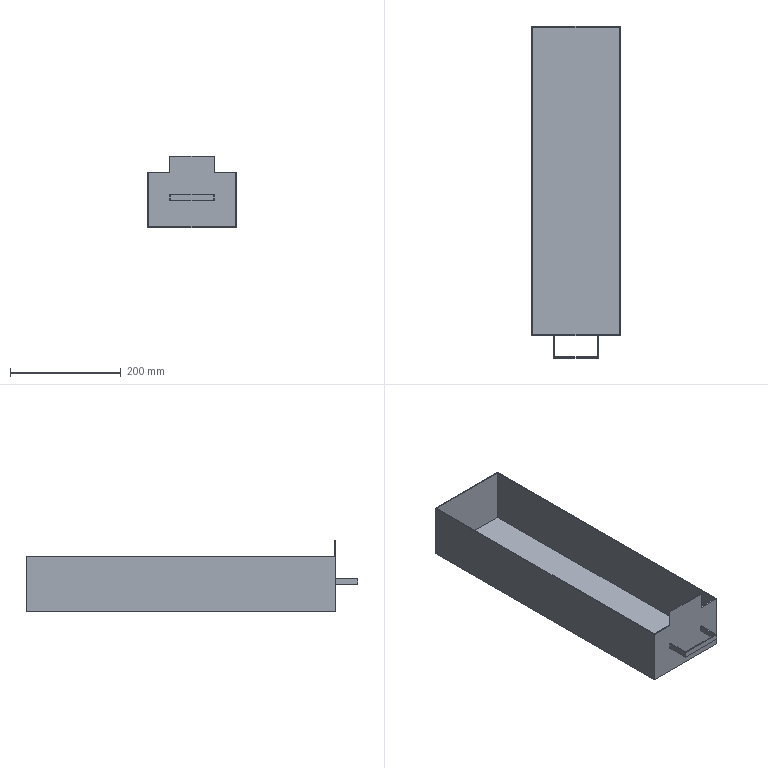Part | NX | features solid 2 | 1 solid | 22 faces | box 160 x 600 x 130 mm | volume 467792 mm3 | plane 22
STEP:
#1=CARTESIAN_POINT('',(375.,-427.,-465.));
#2=VERTEX_POINT('',#1);
#3=CARTESIAN_POINT('',(375.,-987.,-465.));
#4=VERTEX_POINT('',#3);
#5=CARTESIAN_POINT('',(375.,-687.,-465.));
#6=DIRECTION('',(0.,-1.,0.));
#7=VECTOR('',#6,1000.);
#8=LINE('',#5,#7);
#9=EDGE_CURVE('',#2,#4,#8,.T.);
#10=ORIENTED_EDGE('',*,*,#9,.T.);
#11=CARTESIAN_POINT('',(375.,-987.,-565.));
#12=VERTEX_POINT('',#11);
#13=CARTESIAN_POINT('',(375.,-987.,-565.));
#14=DIRECTION('',(0.,0.,1.));
#15=VECTOR('',#14,1000.);
#16=LINE('',#13,#15);
#17=EDGE_CURVE('',#12,#4,#16,.T.);
#18=ORIENTED_EDGE('',*,*,#17,.F.);
#19=CARTESIAN_POINT('',(375.,-427.,-565.));
#20=VERTEX_POINT('',#19);
#21=CARTESIAN_POINT('',(375.,-687.,-565.));
#22=DIRECTION('',(0.,-1.,0.));
#23=VECTOR('',#22,1000.);
#24=LINE('',#21,#23);
#25=EDGE_CURVE('',#20,#12,#24,.T.);
#26=ORIENTED_EDGE('',*,*,#25,.F.);
#27=CARTESIAN_POINT('',(375.,-427.,-565.));
#28=DIRECTION('',(0.,0.,-1.));
#29=VECTOR('',#28,1000.);
#30=LINE('',#27,#29);
#31=EDGE_CURVE('',#20,#2,#30,.F.);
#32=ORIENTED_EDGE('',*,*,#31,.T.);
#33=EDGE_LOOP('',(#10,#18,#26,#32));
#34=FACE_BOUND('',#33,.T.);
#35=CARTESIAN_POINT('',(375.,-687.,-565.));
#36=DIRECTION('',(-1.,0.,0.));
#37=DIRECTION('',(0.,-1.,0.));
#38=AXIS2_PLACEMENT_3D('',#35,#36,#37);
#39=PLANE('',#38);
#40=ADVANCED_FACE('',(#34),#39,.F.);
#41=CARTESIAN_POINT('',(255.,-987.,-505.));
#42=VERTEX_POINT('',#41);
#43=CARTESIAN_POINT('',(255.,-987.,-515.));
#44=VERTEX_POINT('',#43);
#45=CARTESIAN_POINT('',(255.,-987.,-565.));
#46=DIRECTION('',(0.,0.,-1.));
#47=VECTOR('',#46,1000.);
#48=LINE('',#45,#47);
#49=EDGE_CURVE('',#42,#44,#48,.T.);
#50=ORIENTED_EDGE('',*,*,#49,.F.);
#51=CARTESIAN_POINT('',(257.,-987.,-505.));
#52=VERTEX_POINT('',#51);
#53=CARTESIAN_POINT('',(335.,-987.,-505.));
#54=DIRECTION('',(1.,0.,0.));
#55=VECTOR('',#54,1000.);
#56=LINE('',#53,#55);
#57=EDGE_CURVE('',#52,#42,#56,.F.);
#58=ORIENTED_EDGE('',*,*,#57,.F.);
#59=CARTESIAN_POINT('',(257.,-987.,-515.));
#60=VERTEX_POINT('',#59);
#61=CARTESIAN_POINT('',(257.,-987.,-565.));
#62=DIRECTION('',(0.,0.,-1.));
#63=VECTOR('',#62,1000.);
#64=LINE('',#61,#63);
#65=EDGE_CURVE('',#52,#60,#64,.T.);
#66=ORIENTED_EDGE('',*,*,#65,.T.);
#67=CARTESIAN_POINT('',(335.,-987.,-515.));
#68=DIRECTION('',(1.,0.,0.));
#69=VECTOR('',#68,1000.);
#70=LINE('',#67,#69);
#71=EDGE_CURVE('',#60,#44,#70,.F.);
#72=ORIENTED_EDGE('',*,*,#71,.T.);
#73=EDGE_LOOP('',(#50,#58,#66,#72));
#74=FACE_BOUND('',#73,.T.);
#75=CARTESIAN_POINT('',(333.,-987.,-505.));
#76=VERTEX_POINT('',#75);
#77=CARTESIAN_POINT('',(333.,-987.,-515.));
#78=VERTEX_POINT('',#77);
#79=CARTESIAN_POINT('',(333.,-987.,-565.));
#80=DIRECTION('',(0.,0.,1.));
#81=VECTOR('',#80,1000.);
#82=LINE('',#79,#81);
#83=EDGE_CURVE('',#76,#78,#82,.F.);
#84=ORIENTED_EDGE('',*,*,#83,.F.);
#85=CARTESIAN_POINT('',(335.,-987.,-505.));
#86=VERTEX_POINT('',#85);
#87=CARTESIAN_POINT('',(335.,-987.,-505.));
#88=DIRECTION('',(1.,0.,0.));
#89=VECTOR('',#88,1000.);
#90=LINE('',#87,#89);
#91=EDGE_CURVE('',#86,#76,#90,.F.);
#92=ORIENTED_EDGE('',*,*,#91,.F.);
#93=CARTESIAN_POINT('',(335.,-987.,-515.));
#94=VERTEX_POINT('',#93);
#95=CARTESIAN_POINT('',(335.,-987.,-565.));
#96=DIRECTION('',(0.,0.,-1.));
#97=VECTOR('',#96,1000.);
#98=LINE('',#95,#97);
#99=EDGE_CURVE('',#86,#94,#98,.T.);
#100=ORIENTED_EDGE('',*,*,#99,.T.);
#101=CARTESIAN_POINT('',(335.,-987.,-515.));
#102=DIRECTION('',(1.,0.,0.));
#103=VECTOR('',#102,1000.);
#104=LINE('',#101,#103);
#105=EDGE_CURVE('',#94,#78,#104,.F.);
#106=ORIENTED_EDGE('',*,*,#105,.T.);
#107=EDGE_LOOP('',(#84,#92,#100,#106));
#108=FACE_BOUND('',#107,.T.);
#109=CARTESIAN_POINT('',(215.,-987.,-465.));
#110=VERTEX_POINT('',#109);
#111=CARTESIAN_POINT('',(255.,-987.,-465.));
#112=VERTEX_POINT('',#111);
#113=CARTESIAN_POINT('',(370.,-987.,-465.));
#114=DIRECTION('',(1.,0.,0.));
#115=VECTOR('',#114,1000.);
#116=LINE('',#113,#115);
#117=EDGE_CURVE('',#110,#112,#116,.T.);
#118=ORIENTED_EDGE('',*,*,#117,.F.);
#119=CARTESIAN_POINT('',(215.,-987.,-565.));
#120=VERTEX_POINT('',#119);
#121=CARTESIAN_POINT('',(215.,-987.,-565.));
#122=DIRECTION('',(0.,0.,-1.));
#123=VECTOR('',#122,1000.);
#124=LINE('',#121,#123);
#125=EDGE_CURVE('',#120,#110,#124,.F.);
#126=ORIENTED_EDGE('',*,*,#125,.F.);
#127=CARTESIAN_POINT('',(370.,-987.,-565.));
#128=DIRECTION('',(-1.,0.,0.));
#129=VECTOR('',#128,1000.);
#130=LINE('',#127,#129);
#131=EDGE_CURVE('',#12,#120,#130,.T.);
#132=ORIENTED_EDGE('',*,*,#131,.F.);
#133=ORIENTED_EDGE('',*,*,#17,.T.);
#134=CARTESIAN_POINT('',(335.,-987.,-465.));
#135=VERTEX_POINT('',#134);
#136=CARTESIAN_POINT('',(370.,-987.,-465.));
#137=DIRECTION('',(1.,0.,0.));
#138=VECTOR('',#137,1000.);
#139=LINE('',#136,#138);
#140=EDGE_CURVE('',#135,#4,#139,.T.);
#141=ORIENTED_EDGE('',*,*,#140,.F.);
#142=CARTESIAN_POINT('',(335.,-987.,-435.));
#143=VERTEX_POINT('',#142);
#144=CARTESIAN_POINT('',(335.,-987.,-565.));
#145=DIRECTION('',(0.,0.,1.));
#146=VECTOR('',#145,1000.);
#147=LINE('',#144,#146);
#148=EDGE_CURVE('',#135,#143,#147,.T.);
#149=ORIENTED_EDGE('',*,*,#148,.T.);
#150=CARTESIAN_POINT('',(255.,-987.,-435.));
#151=VERTEX_POINT('',#150);
#152=CARTESIAN_POINT('',(375.,-987.,-435.));
#153=DIRECTION('',(-1.,0.,0.));
#154=VECTOR('',#153,1000.);
#155=LINE('',#152,#154);
#156=EDGE_CURVE('',#143,#151,#155,.T.);
#157=ORIENTED_EDGE('',*,*,#156,.T.);
#158=CARTESIAN_POINT('',(255.,-987.,-565.));
#159=DIRECTION('',(0.,0.,-1.));
#160=VECTOR('',#159,1000.);
#161=LINE('',#158,#160);
#162=EDGE_CURVE('',#112,#151,#161,.F.);
#163=ORIENTED_EDGE('',*,*,#162,.F.);
#164=EDGE_LOOP('',(#118,#126,#132,#133,#141,#149,#157,#163));
#165=FACE_BOUND('',#164,.T.);
#166=CARTESIAN_POINT('',(370.,-987.,-565.));
#167=DIRECTION('',(0.,1.,0.));
#168=DIRECTION('',(-1.,0.,0.));
#169=AXIS2_PLACEMENT_3D('',#166,#167,#168);
#170=PLANE('',#169);
#171=ADVANCED_FACE('',(#74,#108,#165),#170,.F.);
#172=ORIENTED_EDGE('',*,*,#125,.T.);
#173=CARTESIAN_POINT('',(215.,-427.,-465.));
#174=VERTEX_POINT('',#173);
#175=CARTESIAN_POINT('',(215.,-687.,-465.));
#176=DIRECTION('',(0.,1.,0.));
#177=VECTOR('',#176,1000.);
#178=LINE('',#175,#177);
#179=EDGE_CURVE('',#174,#110,#178,.F.);
#180=ORIENTED_EDGE('',*,*,#179,.F.);
#181=CARTESIAN_POINT('',(215.,-427.,-565.));
#182=VERTEX_POINT('',#181);
#183=CARTESIAN_POINT('',(215.,-427.,-565.));
#184=DIRECTION('',(0.,0.,1.));
#185=VECTOR('',#184,1000.);
#186=LINE('',#183,#185);
#187=EDGE_CURVE('',#182,#174,#186,.T.);
#188=ORIENTED_EDGE('',*,*,#187,.F.);
#189=CARTESIAN_POINT('',(215.,-687.,-565.));
#190=DIRECTION('',(0.,1.,0.));
#191=VECTOR('',#190,1000.);
#192=LINE('',#189,#191);
#193=EDGE_CURVE('',#182,#120,#192,.F.);
#194=ORIENTED_EDGE('',*,*,#193,.T.);
#195=EDGE_LOOP('',(#172,#180,#188,#194));
#196=FACE_BOUND('',#195,.T.);
#197=CARTESIAN_POINT('',(215.,-687.,-565.));
#198=DIRECTION('',(-1.,0.,0.));
#199=DIRECTION('',(0.,-1.,0.));
#200=AXIS2_PLACEMENT_3D('',#197,#198,#199);
#201=PLANE('',#200);
#202=ADVANCED_FACE('',(#196),#201,.T.);
#203=CARTESIAN_POINT('',(217.,-985.,-563.));
#204=VERTEX_POINT('',#203);
#205=CARTESIAN_POINT('',(217.,-985.,-465.));
#206=VERTEX_POINT('',#205);
#207=CARTESIAN_POINT('',(217.,-985.,-565.));
#208=DIRECTION('',(0.,0.,-1.));
#209=VECTOR('',#208,1000.);
#210=LINE('',#207,#209);
#211=EDGE_CURVE('',#204,#206,#210,.F.);
#212=ORIENTED_EDGE('',*,*,#211,.T.);
#213=CARTESIAN_POINT('',(255.,-985.,-465.));
#214=VERTEX_POINT('',#213);
#215=CARTESIAN_POINT('',(370.,-985.,-465.));
#216=DIRECTION('',(1.,0.,0.));
#217=VECTOR('',#216,1000.);
#218=LINE('',#215,#217);
#219=EDGE_CURVE('',#206,#214,#218,.T.);
#220=ORIENTED_EDGE('',*,*,#219,.T.);
#221=CARTESIAN_POINT('',(255.,-985.,-435.));
#222=VERTEX_POINT('',#221);
#223=CARTESIAN_POINT('',(255.,-985.,-565.));
#224=DIRECTION('',(0.,0.,-1.));
#225=VECTOR('',#224,1000.);
#226=LINE('',#223,#225);
#227=EDGE_CURVE('',#214,#222,#226,.F.);
#228=ORIENTED_EDGE('',*,*,#227,.T.);
#229=CARTESIAN_POINT('',(335.,-985.,-435.));
#230=VERTEX_POINT('',#229);
#231=CARTESIAN_POINT('',(375.,-985.,-435.));
#232=DIRECTION('',(-1.,0.,0.));
#233=VECTOR('',#232,1000.);
#234=LINE('',#231,#233);
#235=EDGE_CURVE('',#230,#222,#234,.T.);
#236=ORIENTED_EDGE('',*,*,#235,.F.);
#237=CARTESIAN_POINT('',(335.,-985.,-465.));
#238=VERTEX_POINT('',#237);
#239=CARTESIAN_POINT('',(335.,-985.,-565.));
#240=DIRECTION('',(0.,0.,1.));
#241=VECTOR('',#240,1000.);
#242=LINE('',#239,#241);
#243=EDGE_CURVE('',#238,#230,#242,.T.);
#244=ORIENTED_EDGE('',*,*,#243,.F.);
#245=CARTESIAN_POINT('',(373.,-985.,-465.));
#246=VERTEX_POINT('',#245);
#247=CARTESIAN_POINT('',(370.,-985.,-465.));
#248=DIRECTION('',(1.,0.,0.));
#249=VECTOR('',#248,1000.);
#250=LINE('',#247,#249);
#251=EDGE_CURVE('',#238,#246,#250,.T.);
#252=ORIENTED_EDGE('',*,*,#251,.T.);
#253=CARTESIAN_POINT('',(373.,-985.,-563.));
#254=VERTEX_POINT('',#253);
#255=CARTESIAN_POINT('',(373.,-985.,-565.));
#256=DIRECTION('',(0.,0.,1.));
#257=VECTOR('',#256,1000.);
#258=LINE('',#255,#257);
#259=EDGE_CURVE('',#254,#246,#258,.T.);
#260=ORIENTED_EDGE('',*,*,#259,.F.);
#261=CARTESIAN_POINT('',(370.,-985.,-563.));
#262=DIRECTION('',(-1.,0.,0.));
#263=VECTOR('',#262,1000.);
#264=LINE('',#261,#263);
#265=EDGE_CURVE('',#254,#204,#264,.T.);
#266=ORIENTED_EDGE('',*,*,#265,.T.);
#267=EDGE_LOOP('',(#212,#220,#228,#236,#244,#252,#260,#266));
#268=FACE_BOUND('',#267,.T.);
#269=CARTESIAN_POINT('',(370.,-985.,-565.));
#270=DIRECTION('',(0.,1.,0.));
#271=DIRECTION('',(-1.,0.,0.));
#272=AXIS2_PLACEMENT_3D('',#269,#270,#271);
#273=PLANE('',#272);
#274=ADVANCED_FACE('',(#268),#273,.T.);
#275=CARTESIAN_POINT('',(255.,-687.,-465.));
#276=DIRECTION('',(0.,1.,0.));
#277=VECTOR('',#276,1000.);
#278=LINE('',#275,#277);
#279=EDGE_CURVE('',#214,#112,#278,.F.);
#280=ORIENTED_EDGE('',*,*,#279,.F.);
#281=ORIENTED_EDGE('',*,*,#219,.F.);
#282=CARTESIAN_POINT('',(217.,-429.,-465.));
#283=VERTEX_POINT('',#282);
#284=CARTESIAN_POINT('',(217.,-687.,-465.));
#285=DIRECTION('',(0.,1.,0.));
#286=VECTOR('',#285,1000.);
#287=LINE('',#284,#286);
#288=EDGE_CURVE('',#283,#206,#287,.F.);
#289=ORIENTED_EDGE('',*,*,#288,.F.);
#290=CARTESIAN_POINT('',(373.,-429.,-465.));
#291=VERTEX_POINT('',#290);
#292=CARTESIAN_POINT('',(370.,-429.,-465.));
#293=DIRECTION('',(1.,0.,0.));
#294=VECTOR('',#293,1000.);
#295=LINE('',#292,#294);
#296=EDGE_CURVE('',#291,#283,#295,.F.);
#297=ORIENTED_EDGE('',*,*,#296,.F.);
#298=CARTESIAN_POINT('',(373.,-687.,-465.));
#299=DIRECTION('',(0.,-1.,0.));
#300=VECTOR('',#299,1000.);
#301=LINE('',#298,#300);
#302=EDGE_CURVE('',#291,#246,#301,.T.);
#303=ORIENTED_EDGE('',*,*,#302,.T.);
#304=ORIENTED_EDGE('',*,*,#251,.F.);
#305=CARTESIAN_POINT('',(335.,-687.,-465.));
#306=DIRECTION('',(0.,1.,0.));
#307=VECTOR('',#306,1000.);
#308=LINE('',#305,#307);
#309=EDGE_CURVE('',#135,#238,#308,.T.);
#310=ORIENTED_EDGE('',*,*,#309,.F.);
#311=ORIENTED_EDGE('',*,*,#140,.T.);
#312=ORIENTED_EDGE('',*,*,#9,.F.);
#313=CARTESIAN_POINT('',(370.,-427.,-465.));
#314=DIRECTION('',(1.,0.,0.));
#315=VECTOR('',#314,1000.);
#316=LINE('',#313,#315);
#317=EDGE_CURVE('',#2,#174,#316,.F.);
#318=ORIENTED_EDGE('',*,*,#317,.T.);
#319=ORIENTED_EDGE('',*,*,#179,.T.);
#320=ORIENTED_EDGE('',*,*,#117,.T.);
#321=EDGE_LOOP('',(#280,#281,#289,#297,#303,#304,#310,#311,#312,#318,#319,#320));
#322=FACE_BOUND('',#321,.T.);
#323=CARTESIAN_POINT('',(370.,-687.,-465.));
#324=DIRECTION('',(0.,0.,1.));
#325=DIRECTION('',(1.,0.,0.));
#326=AXIS2_PLACEMENT_3D('',#323,#324,#325);
#327=PLANE('',#326);
#328=ADVANCED_FACE('',(#322),#327,.T.);
#329=ORIENTED_EDGE('',*,*,#187,.T.);
#330=ORIENTED_EDGE('',*,*,#317,.F.);
#331=ORIENTED_EDGE('',*,*,#31,.F.);
#332=CARTESIAN_POINT('',(370.,-427.,-565.));
#333=DIRECTION('',(1.,0.,0.));
#334=VECTOR('',#333,1000.);
#335=LINE('',#332,#334);
#336=EDGE_CURVE('',#20,#182,#335,.F.);
#337=ORIENTED_EDGE('',*,*,#336,.T.);
#338=EDGE_LOOP('',(#329,#330,#331,#337));
#339=FACE_BOUND('',#338,.T.);
#340=CARTESIAN_POINT('',(370.,-427.,-565.));
#341=DIRECTION('',(0.,1.,0.));
#342=DIRECTION('',(-1.,0.,0.));
#343=AXIS2_PLACEMENT_3D('',#340,#341,#342);
#344=PLANE('',#343);
#345=ADVANCED_FACE('',(#339),#344,.T.);
#346=ORIENTED_EDGE('',*,*,#131,.T.);
#347=ORIENTED_EDGE('',*,*,#193,.F.);
#348=ORIENTED_EDGE('',*,*,#336,.F.);
#349=ORIENTED_EDGE('',*,*,#25,.T.);
#350=EDGE_LOOP('',(#346,#347,#348,#349));
#351=FACE_BOUND('',#350,.T.);
#352=CARTESIAN_POINT('',(370.,-687.,-565.));
#353=DIRECTION('',(0.,0.,1.));
#354=DIRECTION('',(1.,0.,0.));
#355=AXIS2_PLACEMENT_3D('',#352,#353,#354);
#356=PLANE('',#355);
#357=ADVANCED_FACE('',(#351),#356,.F.);
#358=CARTESIAN_POINT('',(217.,-429.,-563.));
#359=VERTEX_POINT('',#358);
#360=CARTESIAN_POINT('',(217.,-429.,-565.));
#361=DIRECTION('',(0.,0.,1.));
#362=VECTOR('',#361,1000.);
#363=LINE('',#360,#362);
#364=EDGE_CURVE('',#359,#283,#363,.T.);
#365=ORIENTED_EDGE('',*,*,#364,.F.);
#366=CARTESIAN_POINT('',(373.,-429.,-563.));
#367=VERTEX_POINT('',#366);
#368=CARTESIAN_POINT('',(370.,-429.,-563.));
#369=DIRECTION('',(1.,0.,0.));
#370=VECTOR('',#369,1000.);
#371=LINE('',#368,#370);
#372=EDGE_CURVE('',#367,#359,#371,.F.);
#373=ORIENTED_EDGE('',*,*,#372,.F.);
#374=CARTESIAN_POINT('',(373.,-429.,-565.));
#375=DIRECTION('',(0.,0.,-1.));
#376=VECTOR('',#375,1000.);
#377=LINE('',#374,#376);
#378=EDGE_CURVE('',#367,#291,#377,.F.);
#379=ORIENTED_EDGE('',*,*,#378,.T.);
#380=ORIENTED_EDGE('',*,*,#296,.T.);
#381=EDGE_LOOP('',(#365,#373,#379,#380));
#382=FACE_BOUND('',#381,.T.);
#383=CARTESIAN_POINT('',(370.,-429.,-565.));
#384=DIRECTION('',(0.,1.,0.));
#385=DIRECTION('',(-1.,0.,0.));
#386=AXIS2_PLACEMENT_3D('',#383,#384,#385);
#387=PLANE('',#386);
#388=ADVANCED_FACE('',(#382),#387,.F.);
#389=ORIENTED_EDGE('',*,*,#378,.F.);
#390=CARTESIAN_POINT('',(373.,-687.,-563.));
#391=DIRECTION('',(0.,-1.,0.));
#392=VECTOR('',#391,1000.);
#393=LINE('',#390,#392);
#394=EDGE_CURVE('',#367,#254,#393,.T.);
#395=ORIENTED_EDGE('',*,*,#394,.T.);
#396=ORIENTED_EDGE('',*,*,#259,.T.);
#397=ORIENTED_EDGE('',*,*,#302,.F.);
#398=EDGE_LOOP('',(#389,#395,#396,#397));
#399=FACE_BOUND('',#398,.T.);
#400=CARTESIAN_POINT('',(373.,-687.,-565.));
#401=DIRECTION('',(-1.,0.,0.));
#402=DIRECTION('',(0.,-1.,0.));
#403=AXIS2_PLACEMENT_3D('',#400,#401,#402);
#404=PLANE('',#403);
#405=ADVANCED_FACE('',(#399),#404,.T.);
#406=CARTESIAN_POINT('',(217.,-687.,-563.));
#407=DIRECTION('',(0.,1.,0.));
#408=VECTOR('',#407,1000.);
#409=LINE('',#406,#408);
#410=EDGE_CURVE('',#359,#204,#409,.F.);
#411=ORIENTED_EDGE('',*,*,#410,.F.);
#412=ORIENTED_EDGE('',*,*,#364,.T.);
#413=ORIENTED_EDGE('',*,*,#288,.T.);
#414=ORIENTED_EDGE('',*,*,#211,.F.);
#415=EDGE_LOOP('',(#411,#412,#413,#414));
#416=FACE_BOUND('',#415,.T.);
#417=CARTESIAN_POINT('',(217.,-687.,-565.));
#418=DIRECTION('',(-1.,0.,0.));
#419=DIRECTION('',(0.,-1.,0.));
#420=AXIS2_PLACEMENT_3D('',#417,#418,#419);
#421=PLANE('',#420);
#422=ADVANCED_FACE('',(#416),#421,.F.);
#423=ORIENTED_EDGE('',*,*,#265,.F.);
#424=ORIENTED_EDGE('',*,*,#394,.F.);
#425=ORIENTED_EDGE('',*,*,#372,.T.);
#426=ORIENTED_EDGE('',*,*,#410,.T.);
#427=EDGE_LOOP('',(#423,#424,#425,#426));
#428=FACE_BOUND('',#427,.T.);
#429=CARTESIAN_POINT('',(370.,-687.,-563.));
#430=DIRECTION('',(0.,0.,1.));
#431=DIRECTION('',(1.,0.,0.));
#432=AXIS2_PLACEMENT_3D('',#429,#430,#431);
#433=PLANE('',#432);
#434=ADVANCED_FACE('',(#428),#433,.T.);
#435=ORIENTED_EDGE('',*,*,#91,.T.);
#436=CARTESIAN_POINT('',(333.,-1025.,-505.));
#437=VERTEX_POINT('',#436);
#438=CARTESIAN_POINT('',(333.,-987.,-505.));
#439=DIRECTION('',(0.,1.,0.));
#440=VECTOR('',#439,1000.);
#441=LINE('',#438,#440);
#442=EDGE_CURVE('',#76,#437,#441,.F.);
#443=ORIENTED_EDGE('',*,*,#442,.T.);
#444=CARTESIAN_POINT('',(257.,-1025.,-505.));
#445=VERTEX_POINT('',#444);
#446=CARTESIAN_POINT('',(335.,-1025.,-505.));
#447=DIRECTION('',(1.,0.,0.));
#448=VECTOR('',#447,1000.);
#449=LINE('',#446,#448);
#450=EDGE_CURVE('',#437,#445,#449,.F.);
#451=ORIENTED_EDGE('',*,*,#450,.T.);
#452=CARTESIAN_POINT('',(257.,-987.,-505.));
#453=DIRECTION('',(0.,-1.,0.));
#454=VECTOR('',#453,1000.);
#455=LINE('',#452,#454);
#456=EDGE_CURVE('',#52,#445,#455,.T.);
#457=ORIENTED_EDGE('',*,*,#456,.F.);
#458=ORIENTED_EDGE('',*,*,#57,.T.);
#459=CARTESIAN_POINT('',(255.,-1027.,-505.));
#460=VERTEX_POINT('',#459);
#461=CARTESIAN_POINT('',(255.,-987.,-505.));
#462=DIRECTION('',(0.,1.,0.));
#463=VECTOR('',#462,1000.);
#464=LINE('',#461,#463);
#465=EDGE_CURVE('',#42,#460,#464,.F.);
#466=ORIENTED_EDGE('',*,*,#465,.T.);
#467=CARTESIAN_POINT('',(335.,-1027.,-505.));
#468=VERTEX_POINT('',#467);
#469=CARTESIAN_POINT('',(335.,-1027.,-505.));
#470=DIRECTION('',(1.,0.,0.));
#471=VECTOR('',#470,1000.);
#472=LINE('',#469,#471);
#473=EDGE_CURVE('',#468,#460,#472,.F.);
#474=ORIENTED_EDGE('',*,*,#473,.F.);
#475=CARTESIAN_POINT('',(335.,-987.,-505.));
#476=DIRECTION('',(0.,1.,0.));
#477=VECTOR('',#476,1000.);
#478=LINE('',#475,#477);
#479=EDGE_CURVE('',#86,#468,#478,.F.);
#480=ORIENTED_EDGE('',*,*,#479,.F.);
#481=EDGE_LOOP('',(#435,#443,#451,#457,#458,#466,#474,#480));
#482=FACE_BOUND('',#481,.T.);
#483=CARTESIAN_POINT('',(335.,-987.,-505.));
#484=DIRECTION('',(0.,0.,1.));
#485=DIRECTION('',(1.,0.,0.));
#486=AXIS2_PLACEMENT_3D('',#483,#484,#485);
#487=PLANE('',#486);
#488=ADVANCED_FACE('',(#482),#487,.T.);
#489=ORIENTED_EDGE('',*,*,#99,.F.);
#490=ORIENTED_EDGE('',*,*,#479,.T.);
#491=CARTESIAN_POINT('',(335.,-1027.,-515.));
#492=VERTEX_POINT('',#491);
#493=CARTESIAN_POINT('',(335.,-1027.,-565.));
#494=DIRECTION('',(0.,0.,-1.));
#495=VECTOR('',#494,1000.);
#496=LINE('',#493,#495);
#497=EDGE_CURVE('',#468,#492,#496,.T.);
#498=ORIENTED_EDGE('',*,*,#497,.T.);
#499=CARTESIAN_POINT('',(335.,-987.,-515.));
#500=DIRECTION('',(0.,1.,0.));
#501=VECTOR('',#500,1000.);
#502=LINE('',#499,#501);
#503=EDGE_CURVE('',#94,#492,#502,.F.);
#504=ORIENTED_EDGE('',*,*,#503,.F.);
#505=EDGE_LOOP('',(#489,#490,#498,#504));
#506=FACE_BOUND('',#505,.T.);
#507=CARTESIAN_POINT('',(335.,-987.,-565.));
#508=DIRECTION('',(-1.,0.,0.));
#509=DIRECTION('',(0.,-1.,0.));
#510=AXIS2_PLACEMENT_3D('',#507,#508,#509);
#511=PLANE('',#510);
#512=ADVANCED_FACE('',(#506),#511,.F.);
#513=ORIENTED_EDGE('',*,*,#497,.F.);
#514=ORIENTED_EDGE('',*,*,#473,.T.);
#515=CARTESIAN_POINT('',(255.,-1027.,-515.));
#516=VERTEX_POINT('',#515);
#517=CARTESIAN_POINT('',(255.,-1027.,-565.));
#518=DIRECTION('',(0.,0.,-1.));
#519=VECTOR('',#518,1000.);
#520=LINE('',#517,#519);
#521=EDGE_CURVE('',#460,#516,#520,.T.);
#522=ORIENTED_EDGE('',*,*,#521,.T.);
#523=CARTESIAN_POINT('',(335.,-1027.,-515.));
#524=DIRECTION('',(1.,0.,0.));
#525=VECTOR('',#524,1000.);
#526=LINE('',#523,#525);
#527=EDGE_CURVE('',#492,#516,#526,.F.);
#528=ORIENTED_EDGE('',*,*,#527,.F.);
#529=EDGE_LOOP('',(#513,#514,#522,#528));
#530=FACE_BOUND('',#529,.T.);
#531=CARTESIAN_POINT('',(335.,-1027.,-565.));
#532=DIRECTION('',(0.,1.,0.));
#533=DIRECTION('',(-1.,0.,0.));
#534=AXIS2_PLACEMENT_3D('',#531,#532,#533);
#535=PLANE('',#534);
#536=ADVANCED_FACE('',(#530),#535,.F.);
#537=ORIENTED_EDGE('',*,*,#71,.F.);
#538=CARTESIAN_POINT('',(257.,-1025.,-515.));
#539=VERTEX_POINT('',#538);
#540=CARTESIAN_POINT('',(257.,-987.,-515.));
#541=DIRECTION('',(0.,-1.,0.));
#542=VECTOR('',#541,1000.);
#543=LINE('',#540,#542);
#544=EDGE_CURVE('',#60,#539,#543,.T.);
#545=ORIENTED_EDGE('',*,*,#544,.T.);
#546=CARTESIAN_POINT('',(333.,-1025.,-515.));
#547=VERTEX_POINT('',#546);
#548=CARTESIAN_POINT('',(335.,-1025.,-515.));
#549=DIRECTION('',(1.,0.,0.));
#550=VECTOR('',#549,1000.);
#551=LINE('',#548,#550);
#552=EDGE_CURVE('',#547,#539,#551,.F.);
#553=ORIENTED_EDGE('',*,*,#552,.F.);
#554=CARTESIAN_POINT('',(333.,-987.,-515.));
#555=DIRECTION('',(0.,1.,0.));
#556=VECTOR('',#555,1000.);
#557=LINE('',#554,#556);
#558=EDGE_CURVE('',#78,#547,#557,.F.);
#559=ORIENTED_EDGE('',*,*,#558,.F.);
#560=ORIENTED_EDGE('',*,*,#105,.F.);
#561=ORIENTED_EDGE('',*,*,#503,.T.);
#562=ORIENTED_EDGE('',*,*,#527,.T.);
#563=CARTESIAN_POINT('',(255.,-987.,-515.));
#564=DIRECTION('',(0.,1.,0.));
#565=VECTOR('',#564,1000.);
#566=LINE('',#563,#565);
#567=EDGE_CURVE('',#44,#516,#566,.F.);
#568=ORIENTED_EDGE('',*,*,#567,.F.);
#569=EDGE_LOOP('',(#537,#545,#553,#559,#560,#561,#562,#568));
#570=FACE_BOUND('',#569,.T.);
#571=CARTESIAN_POINT('',(335.,-987.,-515.));
#572=DIRECTION('',(0.,0.,1.));
#573=DIRECTION('',(1.,0.,0.));
#574=AXIS2_PLACEMENT_3D('',#571,#572,#573);
#575=PLANE('',#574);
#576=ADVANCED_FACE('',(#570),#575,.F.);
#577=ORIENTED_EDGE('',*,*,#465,.F.);
#578=ORIENTED_EDGE('',*,*,#49,.T.);
#579=ORIENTED_EDGE('',*,*,#567,.T.);
#580=ORIENTED_EDGE('',*,*,#521,.F.);
#581=EDGE_LOOP('',(#577,#578,#579,#580));
#582=FACE_BOUND('',#581,.T.);
#583=CARTESIAN_POINT('',(255.,-987.,-565.));
#584=DIRECTION('',(-1.,0.,0.));
#585=DIRECTION('',(0.,-1.,0.));
#586=AXIS2_PLACEMENT_3D('',#583,#584,#585);
#587=PLANE('',#586);
#588=ADVANCED_FACE('',(#582),#587,.T.);
#589=ORIENTED_EDGE('',*,*,#83,.T.);
#590=ORIENTED_EDGE('',*,*,#558,.T.);
#591=CARTESIAN_POINT('',(333.,-1025.,-565.));
#592=DIRECTION('',(0.,0.,-1.));
#593=VECTOR('',#592,1000.);
#594=LINE('',#591,#593);
#595=EDGE_CURVE('',#437,#547,#594,.T.);
#596=ORIENTED_EDGE('',*,*,#595,.F.);
#597=ORIENTED_EDGE('',*,*,#442,.F.);
#598=EDGE_LOOP('',(#589,#590,#596,#597));
#599=FACE_BOUND('',#598,.T.);
#600=CARTESIAN_POINT('',(333.,-987.,-565.));
#601=DIRECTION('',(-1.,0.,0.));
#602=DIRECTION('',(0.,-1.,0.));
#603=AXIS2_PLACEMENT_3D('',#600,#601,#602);
#604=PLANE('',#603);
#605=ADVANCED_FACE('',(#599),#604,.T.);
#606=ORIENTED_EDGE('',*,*,#595,.T.);
#607=ORIENTED_EDGE('',*,*,#552,.T.);
#608=CARTESIAN_POINT('',(257.,-1025.,-565.));
#609=DIRECTION('',(0.,0.,1.));
#610=VECTOR('',#609,1000.);
#611=LINE('',#608,#610);
#612=EDGE_CURVE('',#445,#539,#611,.F.);
#613=ORIENTED_EDGE('',*,*,#612,.F.);
#614=ORIENTED_EDGE('',*,*,#450,.F.);
#615=EDGE_LOOP('',(#606,#607,#613,#614));
#616=FACE_BOUND('',#615,.T.);
#617=CARTESIAN_POINT('',(335.,-1025.,-565.));
#618=DIRECTION('',(0.,1.,0.));
#619=DIRECTION('',(-1.,0.,0.));
#620=AXIS2_PLACEMENT_3D('',#617,#618,#619);
#621=PLANE('',#620);
#622=ADVANCED_FACE('',(#616),#621,.T.);
#623=ORIENTED_EDGE('',*,*,#456,.T.);
#624=ORIENTED_EDGE('',*,*,#612,.T.);
#625=ORIENTED_EDGE('',*,*,#544,.F.);
#626=ORIENTED_EDGE('',*,*,#65,.F.);
#627=EDGE_LOOP('',(#623,#624,#625,#626));
#628=FACE_BOUND('',#627,.T.);
#629=CARTESIAN_POINT('',(257.,-987.,-565.));
#630=DIRECTION('',(-1.,0.,0.));
#631=DIRECTION('',(0.,-1.,0.));
#632=AXIS2_PLACEMENT_3D('',#629,#630,#631);
#633=PLANE('',#632);
#634=ADVANCED_FACE('',(#628),#633,.F.);
#635=ORIENTED_EDGE('',*,*,#235,.T.);
#636=CARTESIAN_POINT('',(255.,-687.,-435.));
#637=DIRECTION('',(0.,-1.,0.));
#638=VECTOR('',#637,1000.);
#639=LINE('',#636,#638);
#640=EDGE_CURVE('',#151,#222,#639,.F.);
#641=ORIENTED_EDGE('',*,*,#640,.F.);
#642=ORIENTED_EDGE('',*,*,#156,.F.);
#643=CARTESIAN_POINT('',(335.,-987.,-435.));
#644=DIRECTION('',(0.,1.,0.));
#645=VECTOR('',#644,1000.);
#646=LINE('',#643,#645);
#647=EDGE_CURVE('',#143,#230,#646,.T.);
#648=ORIENTED_EDGE('',*,*,#647,.T.);
#649=EDGE_LOOP('',(#635,#641,#642,#648));
#650=FACE_BOUND('',#649,.T.);
#651=CARTESIAN_POINT('',(375.,-987.,-435.));
#652=DIRECTION('',(0.,0.,-1.));
#653=DIRECTION('',(-1.,0.,0.));
#654=AXIS2_PLACEMENT_3D('',#651,#652,#653);
#655=PLANE('',#654);
#656=ADVANCED_FACE('',(#650),#655,.F.);
#657=ORIENTED_EDGE('',*,*,#227,.F.);
#658=ORIENTED_EDGE('',*,*,#279,.T.);
#659=ORIENTED_EDGE('',*,*,#162,.T.);
#660=ORIENTED_EDGE('',*,*,#640,.T.);
#661=EDGE_LOOP('',(#657,#658,#659,#660));
#662=FACE_BOUND('',#661,.T.);
#663=CARTESIAN_POINT('',(255.,-687.,-565.));
#664=DIRECTION('',(-1.,0.,0.));
#665=DIRECTION('',(0.,-1.,0.));
#666=AXIS2_PLACEMENT_3D('',#663,#664,#665);
#667=PLANE('',#666);
#668=ADVANCED_FACE('',(#662),#667,.T.);
#669=ORIENTED_EDGE('',*,*,#148,.F.);
#670=ORIENTED_EDGE('',*,*,#309,.T.);
#671=ORIENTED_EDGE('',*,*,#243,.T.);
#672=ORIENTED_EDGE('',*,*,#647,.F.);
#673=EDGE_LOOP('',(#669,#670,#671,#672));
#674=FACE_BOUND('',#673,.T.);
#675=CARTESIAN_POINT('',(335.,-687.,-565.));
#676=DIRECTION('',(-1.,0.,0.));
#677=DIRECTION('',(0.,-1.,0.));
#678=AXIS2_PLACEMENT_3D('',#675,#676,#677);
#679=PLANE('',#678);
#680=ADVANCED_FACE('',(#674),#679,.F.);
#681=CLOSED_SHELL('',(#40,#171,#202,#274,#328,#345,#357,#388,#405,#422,#434,#488,#512,#536,#576,#588,#605,#622,#634,#656,#668,#680));
#682=MANIFOLD_SOLID_BREP('',#681);
#683=(LENGTH_UNIT()NAMED_UNIT(*)SI_UNIT(.MILLI.,.METRE.));
#684=UNCERTAINTY_MEASURE_WITH_UNIT(LENGTH_MEASURE(0.00001),#683,'','');
#685=(NAMED_UNIT(*)PLANE_ANGLE_UNIT()SI_UNIT($,.RADIAN.));
#686=(NAMED_UNIT(*)SI_UNIT($,.STERADIAN.)SOLID_ANGLE_UNIT());
#687=(GEOMETRIC_REPRESENTATION_CONTEXT(3)GLOBAL_UNCERTAINTY_ASSIGNED_CONTEXT((#684))GLOBAL_UNIT_ASSIGNED_CONTEXT((#683,#685,#686))REPRESENTATION_CONTEXT('',''));
#688=ADVANCED_BREP_SHAPE_REPRESENTATION('',(#682),#687);